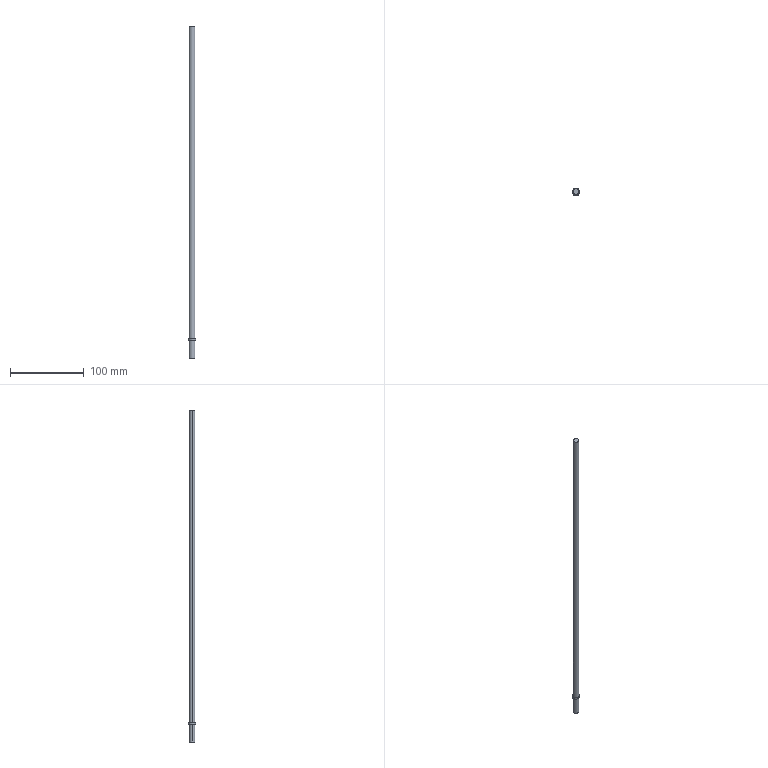Part | SolidWorks | features ICE 8, Extrusion 1 | 1 solid | 22 faces | box 10 x 10 x 449.1 mm | volume 22555 mm3 | cylinder 12 | plane 10 | commonest cylinder face diameters 3 x6 8 x4 10 x2
STEP:
#1=CARTESIAN_POINT('',(0.,2.2,447.1));
#2=VERTEX_POINT('',#1);
#3=CARTESIAN_POINT('',(1.5,2.2,445.6));
#4=VERTEX_POINT('',#3);
#5=CARTESIAN_POINT('',(0.,2.2,445.6));
#6=DIRECTION('',(0.,1.,0.));
#7=DIRECTION('',(0.,0.,1.));
#8=AXIS2_PLACEMENT_3D('',#5,#6,#7);
#9=CIRCLE('',#8,1.5);
#10=EDGE_CURVE('',#2,#4,#9,.T.);
#11=ORIENTED_EDGE('',*,*,#10,.F.);
#12=CARTESIAN_POINT('',(0.,4.,447.1));
#13=VERTEX_POINT('',#12);
#14=CARTESIAN_POINT('',(0.,2.2,447.1));
#15=DIRECTION('',(0.,1.,0.));
#16=VECTOR('',#15,1000.);
#17=LINE('',#14,#16);
#18=EDGE_CURVE('',#2,#13,#17,.T.);
#19=ORIENTED_EDGE('',*,*,#18,.T.);
#20=CARTESIAN_POINT('',(1.5,3.708,445.6));
#21=VERTEX_POINT('',#20);
#22=CARTESIAN_POINT('',(1.5,3.708,445.6));
#23=CARTESIAN_POINT('',(1.5,3.708,445.7));
#24=CARTESIAN_POINT('',(1.49,3.712,445.798));
#25=CARTESIAN_POINT('',(1.451,3.727,445.991));
#26=CARTESIAN_POINT('',(1.422,3.739,446.087));
#27=CARTESIAN_POINT('',(1.309,3.781,446.359));
#28=CARTESIAN_POINT('',(1.197,3.819,446.524));
#29=CARTESIAN_POINT('',(0.9232,3.895,446.798));
#30=CARTESIAN_POINT('',(0.7573,3.932,446.909));
#31=CARTESIAN_POINT('',(0.4867,3.971,447.022));
#32=CARTESIAN_POINT('',(0.3912,3.982,447.051));
#33=CARTESIAN_POINT('',(0.197,3.996,447.09));
#34=CARTESIAN_POINT('',(0.09895,4.,447.1));
#35=CARTESIAN_POINT('',(0.,4.,447.1));
#36=B_SPLINE_CURVE_WITH_KNOTS('',3,(#22,#23,#24,#25,#26,#27,#28,#29,#30,#31,#32,#33,#34,#35),.UNSPECIFIED.,.F.,.F.,(4,2,2,2,2,2,4),(0.,0.0002959,0.0005918,0.001184,0.001775,0.002071,0.002367),.UNSPECIFIED.);
#37=EDGE_CURVE('',#21,#13,#36,.T.);
#38=ORIENTED_EDGE('',*,*,#37,.F.);
#39=CARTESIAN_POINT('',(1.5,2.2,445.6));
#40=DIRECTION('',(0.,1.,0.));
#41=VECTOR('',#40,1000.);
#42=LINE('',#39,#41);
#43=EDGE_CURVE('',#4,#21,#42,.T.);
#44=ORIENTED_EDGE('',*,*,#43,.F.);
#45=EDGE_LOOP('',(#11,#19,#38,#44));
#46=FACE_OUTER_BOUND('',#45,.T.);
#47=CARTESIAN_POINT('',(0.,2.2,445.6));
#48=DIRECTION('',(0.,1.,0.));
#49=DIRECTION('',(0.,0.,1.));
#50=AXIS2_PLACEMENT_3D('',#47,#48,#49);
#51=CYLINDRICAL_SURFACE('',#50,1.5);
#52=ADVANCED_FACE('',(#46),#51,.F.);
#53=CARTESIAN_POINT('',(1.5,3.708,440.6));
#54=VERTEX_POINT('',#53);
#55=CARTESIAN_POINT('',(1.5,3.708,68.));
#56=DIRECTION('',(0.,0.,1.));
#57=VECTOR('',#56,1000.);
#58=LINE('',#55,#57);
#59=EDGE_CURVE('',#54,#21,#58,.T.);
#60=ORIENTED_EDGE('',*,*,#59,.T.);
#61=ORIENTED_EDGE('',*,*,#37,.T.);
#62=CARTESIAN_POINT('',(-1.5,3.708,445.6));
#63=VERTEX_POINT('',#62);
#64=CARTESIAN_POINT('',(0.,4.,447.1));
#65=CARTESIAN_POINT('',(-0.0988,4.,447.1));
#66=CARTESIAN_POINT('',(-0.1991,3.996,447.09));
#67=CARTESIAN_POINT('',(-0.3921,3.982,447.051));
#68=CARTESIAN_POINT('',(-0.486,3.971,447.023));
#69=CARTESIAN_POINT('',(-0.6687,3.945,446.946));
#70=CARTESIAN_POINT('',(-0.7547,3.929,446.9));
#71=CARTESIAN_POINT('',(-0.9162,3.895,446.792));
#72=CARTESIAN_POINT('',(-0.9924,3.876,446.729));
#73=CARTESIAN_POINT('',(-1.13,3.838,446.591));
#74=CARTESIAN_POINT('',(-1.191,3.819,446.517));
#75=CARTESIAN_POINT('',(-1.3,3.783,446.355));
#76=CARTESIAN_POINT('',(-1.347,3.767,446.268));
#77=CARTESIAN_POINT('',(-1.459,3.725,445.998));
#78=CARTESIAN_POINT('',(-1.5,3.708,445.8));
#79=CARTESIAN_POINT('',(-1.5,3.708,445.6));
#80=B_SPLINE_CURVE_WITH_KNOTS('',3,(#64,#65,#66,#67,#68,#69,#70,#71,#72,#73,#74,#75,#76,#77,#78,#79),.UNSPECIFIED.,.F.,.F.,(4,2,2,2,2,2,2,4),(0.002367,0.002663,0.002958,0.003254,0.003549,0.003845,0.00414,0.004731),.UNSPECIFIED.);
#81=EDGE_CURVE('',#13,#63,#80,.T.);
#82=ORIENTED_EDGE('',*,*,#81,.T.);
#83=CARTESIAN_POINT('',(-1.5,3.708,440.6));
#84=VERTEX_POINT('',#83);
#85=CARTESIAN_POINT('',(-1.5,3.708,68.));
#86=DIRECTION('',(0.,0.,-1.));
#87=VECTOR('',#86,1000.);
#88=LINE('',#85,#87);
#89=EDGE_CURVE('',#63,#84,#88,.T.);
#90=ORIENTED_EDGE('',*,*,#89,.T.);
#91=CARTESIAN_POINT('',(-1.5,3.708,440.6));
#92=CARTESIAN_POINT('',(-1.5,3.708,440.5));
#93=CARTESIAN_POINT('',(-1.49,3.712,440.402));
#94=CARTESIAN_POINT('',(-1.451,3.727,440.209));
#95=CARTESIAN_POINT('',(-1.422,3.739,440.113));
#96=CARTESIAN_POINT('',(-1.309,3.781,439.842));
#97=CARTESIAN_POINT('',(-1.198,3.819,439.677));
#98=CARTESIAN_POINT('',(-0.924,3.894,439.403));
#99=CARTESIAN_POINT('',(-0.7582,3.932,439.291));
#100=CARTESIAN_POINT('',(-0.488,3.971,439.178));
#101=CARTESIAN_POINT('',(-0.3926,3.982,439.149));
#102=CARTESIAN_POINT('',(-0.1986,3.996,439.11));
#103=CARTESIAN_POINT('',(-0.1006,4.,439.1));
#104=CARTESIAN_POINT('',(0.09712,4.,439.1));
#105=CARTESIAN_POINT('',(0.1975,3.996,439.11));
#106=CARTESIAN_POINT('',(0.3907,3.982,439.148));
#107=CARTESIAN_POINT('',(0.4847,3.972,439.177));
#108=CARTESIAN_POINT('',(0.759,3.932,439.291));
#109=CARTESIAN_POINT('',(0.9229,3.895,439.402));
#110=CARTESIAN_POINT('',(1.129,3.838,439.608));
#111=CARTESIAN_POINT('',(1.191,3.819,439.683));
#112=CARTESIAN_POINT('',(1.299,3.783,439.844));
#113=CARTESIAN_POINT('',(1.347,3.767,439.932));
#114=CARTESIAN_POINT('',(1.459,3.725,440.202));
#115=CARTESIAN_POINT('',(1.5,3.708,440.4));
#116=CARTESIAN_POINT('',(1.5,3.708,440.6));
#117=B_SPLINE_CURVE_WITH_KNOTS('',3,(#91,#92,#93,#94,#95,#96,#97,#98,#99,#100,#101,#102,#103,#104,#105,#106,#107,#108,#109,#110,#111,#112,#113,#114,#115,#116),.UNSPECIFIED.,.F.,.F.,(4,2,2,2,2,2,2,2,2,2,2,2,4),(0.,0.0002957,0.0005914,0.001183,0.001774,0.00207,0.002366,0.002661,0.002957,0.003548,0.003844,0.00414,0.004731),.UNSPECIFIED.);
#118=EDGE_CURVE('',#84,#54,#117,.T.);
#119=ORIENTED_EDGE('',*,*,#118,.T.);
#120=EDGE_LOOP('',(#60,#61,#82,#90,#119));
#121=FACE_BOUND('',#120,.T.);
#122=CARTESIAN_POINT('',(4.,0.,449.1));
#123=VERTEX_POINT('',#122);
#124=CARTESIAN_POINT('',(-4.,0.,449.1));
#125=VERTEX_POINT('',#124);
#126=CARTESIAN_POINT('',(0.,0.,449.1));
#127=DIRECTION('',(0.,0.,1.));
#128=DIRECTION('',(1.,0.,0.));
#129=AXIS2_PLACEMENT_3D('',#126,#127,#128);
#130=CIRCLE('',#129,4.);
#131=EDGE_CURVE('',#123,#125,#130,.T.);
#132=ORIENTED_EDGE('',*,*,#131,.F.);
#133=CARTESIAN_POINT('',(4.,0.,26.));
#134=VERTEX_POINT('',#133);
#135=CARTESIAN_POINT('',(4.,0.,68.));
#136=DIRECTION('',(0.,0.,-1.));
#137=VECTOR('',#136,1000.);
#138=LINE('',#135,#137);
#139=EDGE_CURVE('',#123,#134,#138,.T.);
#140=ORIENTED_EDGE('',*,*,#139,.T.);
#141=CARTESIAN_POINT('',(-4.,0.,26.));
#142=VERTEX_POINT('',#141);
#143=CARTESIAN_POINT('',(0.,0.,26.));
#144=DIRECTION('',(0.,0.,1.));
#145=DIRECTION('',(1.,0.,0.));
#146=AXIS2_PLACEMENT_3D('',#143,#144,#145);
#147=CIRCLE('',#146,4.);
#148=EDGE_CURVE('',#134,#142,#147,.T.);
#149=ORIENTED_EDGE('',*,*,#148,.T.);
#150=CARTESIAN_POINT('',(-4.,0.,68.));
#151=DIRECTION('',(0.,0.,-1.));
#152=VECTOR('',#151,1000.);
#153=LINE('',#150,#152);
#154=EDGE_CURVE('',#125,#142,#153,.T.);
#155=ORIENTED_EDGE('',*,*,#154,.F.);
#156=EDGE_LOOP('',(#132,#140,#149,#155));
#157=FACE_OUTER_BOUND('',#156,.T.);
#158=CARTESIAN_POINT('',(0.,0.,68.));
#159=DIRECTION('',(0.,0.,-1.));
#160=DIRECTION('',(-1.,0.,0.));
#161=AXIS2_PLACEMENT_3D('',#158,#159,#160);
#162=CYLINDRICAL_SURFACE('',#161,4.);
#163=ADVANCED_FACE('',(#121,#157),#162,.T.);
#164=CARTESIAN_POINT('',(0.,2.2,12.));
#165=VERTEX_POINT('',#164);
#166=CARTESIAN_POINT('',(1.5,2.2,10.5));
#167=VERTEX_POINT('',#166);
#168=CARTESIAN_POINT('',(0.,2.2,10.5));
#169=DIRECTION('',(0.,1.,0.));
#170=DIRECTION('',(0.,0.,1.));
#171=AXIS2_PLACEMENT_3D('',#168,#169,#170);
#172=CIRCLE('',#171,1.5);
#173=EDGE_CURVE('',#165,#167,#172,.T.);
#174=ORIENTED_EDGE('',*,*,#173,.F.);
#175=CARTESIAN_POINT('',(0.,4.,12.));
#176=VERTEX_POINT('',#175);
#177=CARTESIAN_POINT('',(0.,2.2,12.));
#178=DIRECTION('',(0.,1.,0.));
#179=VECTOR('',#178,1000.);
#180=LINE('',#177,#179);
#181=EDGE_CURVE('',#165,#176,#180,.T.);
#182=ORIENTED_EDGE('',*,*,#181,.T.);
#183=CARTESIAN_POINT('',(1.5,3.708,10.5));
#184=VERTEX_POINT('',#183);
#185=CARTESIAN_POINT('',(1.5,3.708,10.5));
#186=CARTESIAN_POINT('',(1.5,3.708,10.6));
#187=CARTESIAN_POINT('',(1.49,3.712,10.698));
#188=CARTESIAN_POINT('',(1.451,3.727,10.891));
#189=CARTESIAN_POINT('',(1.422,3.739,10.987));
#190=CARTESIAN_POINT('',(1.309,3.781,11.259));
#191=CARTESIAN_POINT('',(1.197,3.819,11.424));
#192=CARTESIAN_POINT('',(0.9232,3.895,11.698));
#193=CARTESIAN_POINT('',(0.7573,3.932,11.809));
#194=CARTESIAN_POINT('',(0.4867,3.971,11.922));
#195=CARTESIAN_POINT('',(0.3912,3.982,11.951));
#196=CARTESIAN_POINT('',(0.197,3.996,11.99));
#197=CARTESIAN_POINT('',(0.09895,4.,12.));
#198=CARTESIAN_POINT('',(0.,4.,12.));
#199=B_SPLINE_CURVE_WITH_KNOTS('',3,(#185,#186,#187,#188,#189,#190,#191,#192,#193,#194,#195,#196,#197,#198),.UNSPECIFIED.,.F.,.F.,(4,2,2,2,2,2,4),(0.,0.0002959,0.0005918,0.001184,0.001775,0.002071,0.002367),.UNSPECIFIED.);
#200=EDGE_CURVE('',#184,#176,#199,.T.);
#201=ORIENTED_EDGE('',*,*,#200,.F.);
#202=CARTESIAN_POINT('',(1.5,2.2,10.5));
#203=DIRECTION('',(0.,1.,0.));
#204=VECTOR('',#203,1000.);
#205=LINE('',#202,#204);
#206=EDGE_CURVE('',#167,#184,#205,.T.);
#207=ORIENTED_EDGE('',*,*,#206,.F.);
#208=EDGE_LOOP('',(#174,#182,#201,#207));
#209=FACE_OUTER_BOUND('',#208,.T.);
#210=CARTESIAN_POINT('',(0.,2.2,10.5));
#211=DIRECTION('',(0.,1.,0.));
#212=DIRECTION('',(0.,0.,1.));
#213=AXIS2_PLACEMENT_3D('',#210,#211,#212);
#214=CYLINDRICAL_SURFACE('',#213,1.5);
#215=ADVANCED_FACE('',(#209),#214,.F.);
#216=CARTESIAN_POINT('',(5.,0.,26.));
#217=VERTEX_POINT('',#216);
#218=CARTESIAN_POINT('',(-5.,0.,26.));
#219=VERTEX_POINT('',#218);
#220=CARTESIAN_POINT('',(0.,0.,26.));
#221=DIRECTION('',(0.,0.,1.));
#222=DIRECTION('',(1.,0.,0.));
#223=AXIS2_PLACEMENT_3D('',#220,#221,#222);
#224=CIRCLE('',#223,5.);
#225=EDGE_CURVE('',#217,#219,#224,.T.);
#226=ORIENTED_EDGE('',*,*,#225,.F.);
#227=CARTESIAN_POINT('',(5.,0.,24.));
#228=VERTEX_POINT('',#227);
#229=CARTESIAN_POINT('',(5.,0.,26.));
#230=DIRECTION('',(0.,0.,-1.));
#231=VECTOR('',#230,1000.);
#232=LINE('',#229,#231);
#233=EDGE_CURVE('',#217,#228,#232,.T.);
#234=ORIENTED_EDGE('',*,*,#233,.T.);
#235=CARTESIAN_POINT('',(-5.,0.,24.));
#236=VERTEX_POINT('',#235);
#237=CARTESIAN_POINT('',(0.,0.,24.));
#238=DIRECTION('',(0.,0.,1.));
#239=DIRECTION('',(1.,0.,0.));
#240=AXIS2_PLACEMENT_3D('',#237,#238,#239);
#241=CIRCLE('',#240,5.);
#242=EDGE_CURVE('',#228,#236,#241,.T.);
#243=ORIENTED_EDGE('',*,*,#242,.T.);
#244=CARTESIAN_POINT('',(-5.,0.,26.));
#245=DIRECTION('',(0.,0.,-1.));
#246=VECTOR('',#245,1000.);
#247=LINE('',#244,#246);
#248=EDGE_CURVE('',#219,#236,#247,.T.);
#249=ORIENTED_EDGE('',*,*,#248,.F.);
#250=EDGE_LOOP('',(#226,#234,#243,#249));
#251=FACE_OUTER_BOUND('',#250,.T.);
#252=CARTESIAN_POINT('',(0.,0.,26.));
#253=DIRECTION('',(0.,0.,-1.));
#254=DIRECTION('',(-1.,0.,0.));
#255=AXIS2_PLACEMENT_3D('',#252,#253,#254);
#256=CYLINDRICAL_SURFACE('',#255,5.);
#257=ADVANCED_FACE('',(#251),#256,.T.);
#258=CARTESIAN_POINT('',(1.5,3.708,5.5));
#259=VERTEX_POINT('',#258);
#260=CARTESIAN_POINT('',(1.5,3.708,14.));
#261=DIRECTION('',(0.,0.,1.));
#262=VECTOR('',#261,1000.);
#263=LINE('',#260,#262);
#264=EDGE_CURVE('',#259,#184,#263,.T.);
#265=ORIENTED_EDGE('',*,*,#264,.T.);
#266=ORIENTED_EDGE('',*,*,#200,.T.);
#267=CARTESIAN_POINT('',(-1.5,3.708,10.5));
#268=VERTEX_POINT('',#267);
#269=CARTESIAN_POINT('',(0.,4.,12.));
#270=CARTESIAN_POINT('',(-0.0988,4.,12.));
#271=CARTESIAN_POINT('',(-0.1991,3.996,11.99));
#272=CARTESIAN_POINT('',(-0.3921,3.982,11.951));
#273=CARTESIAN_POINT('',(-0.486,3.971,11.923));
#274=CARTESIAN_POINT('',(-0.6687,3.945,11.846));
#275=CARTESIAN_POINT('',(-0.7547,3.929,11.8));
#276=CARTESIAN_POINT('',(-0.9162,3.895,11.692));
#277=CARTESIAN_POINT('',(-0.9924,3.876,11.629));
#278=CARTESIAN_POINT('',(-1.13,3.838,11.491));
#279=CARTESIAN_POINT('',(-1.191,3.819,11.417));
#280=CARTESIAN_POINT('',(-1.3,3.783,11.255));
#281=CARTESIAN_POINT('',(-1.347,3.767,11.168));
#282=CARTESIAN_POINT('',(-1.459,3.725,10.898));
#283=CARTESIAN_POINT('',(-1.5,3.708,10.7));
#284=CARTESIAN_POINT('',(-1.5,3.708,10.5));
#285=B_SPLINE_CURVE_WITH_KNOTS('',3,(#269,#270,#271,#272,#273,#274,#275,#276,#277,#278,#279,#280,#281,#282,#283,#284),.UNSPECIFIED.,.F.,.F.,(4,2,2,2,2,2,2,4),(0.002367,0.002663,0.002958,0.003254,0.003549,0.003845,0.00414,0.004731),.UNSPECIFIED.);
#286=EDGE_CURVE('',#176,#268,#285,.T.);
#287=ORIENTED_EDGE('',*,*,#286,.T.);
#288=CARTESIAN_POINT('',(-1.5,3.708,5.5));
#289=VERTEX_POINT('',#288);
#290=CARTESIAN_POINT('',(-1.5,3.708,14.));
#291=DIRECTION('',(0.,0.,-1.));
#292=VECTOR('',#291,1000.);
#293=LINE('',#290,#292);
#294=EDGE_CURVE('',#268,#289,#293,.T.);
#295=ORIENTED_EDGE('',*,*,#294,.T.);
#296=CARTESIAN_POINT('',(-1.5,3.708,5.5));
#297=CARTESIAN_POINT('',(-1.5,3.708,5.4));
#298=CARTESIAN_POINT('',(-1.49,3.712,5.302));
#299=CARTESIAN_POINT('',(-1.451,3.727,5.109));
#300=CARTESIAN_POINT('',(-1.422,3.739,5.013));
#301=CARTESIAN_POINT('',(-1.309,3.781,4.742));
#302=CARTESIAN_POINT('',(-1.198,3.819,4.577));
#303=CARTESIAN_POINT('',(-0.924,3.894,4.303));
#304=CARTESIAN_POINT('',(-0.7582,3.932,4.191));
#305=CARTESIAN_POINT('',(-0.488,3.971,4.078));
#306=CARTESIAN_POINT('',(-0.3926,3.982,4.049));
#307=CARTESIAN_POINT('',(-0.1986,3.996,4.01));
#308=CARTESIAN_POINT('',(-0.1006,4.,4.));
#309=CARTESIAN_POINT('',(0.09712,4.,4.));
#310=CARTESIAN_POINT('',(0.1975,3.996,4.01));
#311=CARTESIAN_POINT('',(0.3907,3.982,4.048));
#312=CARTESIAN_POINT('',(0.4847,3.972,4.077));
#313=CARTESIAN_POINT('',(0.759,3.932,4.191));
#314=CARTESIAN_POINT('',(0.9229,3.895,4.302));
#315=CARTESIAN_POINT('',(1.129,3.838,4.508));
#316=CARTESIAN_POINT('',(1.191,3.819,4.583));
#317=CARTESIAN_POINT('',(1.299,3.783,4.744));
#318=CARTESIAN_POINT('',(1.347,3.767,4.832));
#319=CARTESIAN_POINT('',(1.459,3.725,5.102));
#320=CARTESIAN_POINT('',(1.5,3.708,5.3));
#321=CARTESIAN_POINT('',(1.5,3.708,5.5));
#322=B_SPLINE_CURVE_WITH_KNOTS('',3,(#296,#297,#298,#299,#300,#301,#302,#303,#304,#305,#306,#307,#308,#309,#310,#311,#312,#313,#314,#315,#316,#317,#318,#319,#320,#321),.UNSPECIFIED.,.F.,.F.,(4,2,2,2,2,2,2,2,2,2,2,2,4),(0.,0.0002957,0.0005914,0.001183,0.001774,0.00207,0.002366,0.002661,0.002957,0.003548,0.003844,0.00414,0.004731),.UNSPECIFIED.);
#323=EDGE_CURVE('',#289,#259,#322,.T.);
#324=ORIENTED_EDGE('',*,*,#323,.T.);
#325=EDGE_LOOP('',(#265,#266,#287,#295,#324));
#326=FACE_BOUND('',#325,.T.);
#327=CARTESIAN_POINT('',(4.,0.,24.));
#328=VERTEX_POINT('',#327);
#329=CARTESIAN_POINT('',(-4.,0.,24.));
#330=VERTEX_POINT('',#329);
#331=CARTESIAN_POINT('',(0.,0.,24.));
#332=DIRECTION('',(0.,0.,1.));
#333=DIRECTION('',(1.,0.,0.));
#334=AXIS2_PLACEMENT_3D('',#331,#332,#333);
#335=CIRCLE('',#334,4.);
#336=EDGE_CURVE('',#328,#330,#335,.T.);
#337=ORIENTED_EDGE('',*,*,#336,.F.);
#338=CARTESIAN_POINT('',(4.,0.,0.));
#339=VERTEX_POINT('',#338);
#340=CARTESIAN_POINT('',(4.,0.,14.));
#341=DIRECTION('',(0.,0.,-1.));
#342=VECTOR('',#341,1000.);
#343=LINE('',#340,#342);
#344=EDGE_CURVE('',#328,#339,#343,.T.);
#345=ORIENTED_EDGE('',*,*,#344,.T.);
#346=CARTESIAN_POINT('',(-4.,0.,0.));
#347=VERTEX_POINT('',#346);
#348=CARTESIAN_POINT('',(0.,0.,0.));
#349=DIRECTION('',(0.,0.,1.));
#350=DIRECTION('',(1.,0.,0.));
#351=AXIS2_PLACEMENT_3D('',#348,#349,#350);
#352=CIRCLE('',#351,4.);
#353=EDGE_CURVE('',#339,#347,#352,.T.);
#354=ORIENTED_EDGE('',*,*,#353,.T.);
#355=CARTESIAN_POINT('',(-4.,0.,14.));
#356=DIRECTION('',(0.,0.,-1.));
#357=VECTOR('',#356,1000.);
#358=LINE('',#355,#357);
#359=EDGE_CURVE('',#330,#347,#358,.T.);
#360=ORIENTED_EDGE('',*,*,#359,.F.);
#361=EDGE_LOOP('',(#337,#345,#354,#360));
#362=FACE_OUTER_BOUND('',#361,.T.);
#363=CARTESIAN_POINT('',(0.,0.,14.));
#364=DIRECTION('',(0.,0.,-1.));
#365=DIRECTION('',(-1.,0.,0.));
#366=AXIS2_PLACEMENT_3D('',#363,#364,#365);
#367=CYLINDRICAL_SURFACE('',#366,4.);
#368=ADVANCED_FACE('',(#326,#362),#367,.T.);
#369=ORIENTED_EDGE('',*,*,#344,.F.);
#370=CARTESIAN_POINT('',(0.,0.,24.));
#371=DIRECTION('',(0.,0.,1.));
#372=DIRECTION('',(1.,0.,0.));
#373=AXIS2_PLACEMENT_3D('',#370,#371,#372);
#374=CIRCLE('',#373,4.);
#375=EDGE_CURVE('',#330,#328,#374,.T.);
#376=ORIENTED_EDGE('',*,*,#375,.F.);
#377=ORIENTED_EDGE('',*,*,#359,.T.);
#378=CARTESIAN_POINT('',(0.,0.,0.));
#379=DIRECTION('',(0.,0.,1.));
#380=DIRECTION('',(1.,0.,0.));
#381=AXIS2_PLACEMENT_3D('',#378,#379,#380);
#382=CIRCLE('',#381,4.);
#383=EDGE_CURVE('',#347,#339,#382,.T.);
#384=ORIENTED_EDGE('',*,*,#383,.T.);
#385=EDGE_LOOP('',(#369,#376,#377,#384));
#386=FACE_OUTER_BOUND('',#385,.T.);
#387=CARTESIAN_POINT('',(0.,0.,14.));
#388=DIRECTION('',(0.,0.,-1.));
#389=DIRECTION('',(-1.,0.,0.));
#390=AXIS2_PLACEMENT_3D('',#387,#388,#389);
#391=CYLINDRICAL_SURFACE('',#390,4.);
#392=ADVANCED_FACE('',(#386),#391,.T.);
#393=ORIENTED_EDGE('',*,*,#383,.F.);
#394=ORIENTED_EDGE('',*,*,#353,.F.);
#395=EDGE_LOOP('',(#393,#394));
#396=FACE_OUTER_BOUND('',#395,.T.);
#397=CARTESIAN_POINT('',(0.,0.,0.));
#398=DIRECTION('',(0.,0.,1.));
#399=DIRECTION('',(1.,0.,0.));
#400=AXIS2_PLACEMENT_3D('',#397,#398,#399);
#401=PLANE('',#400);
#402=ADVANCED_FACE('',(#396),#401,.F.);
#403=ORIENTED_EDGE('',*,*,#233,.F.);
#404=CARTESIAN_POINT('',(0.,0.,26.));
#405=DIRECTION('',(0.,0.,1.));
#406=DIRECTION('',(1.,0.,0.));
#407=AXIS2_PLACEMENT_3D('',#404,#405,#406);
#408=CIRCLE('',#407,5.);
#409=EDGE_CURVE('',#219,#217,#408,.T.);
#410=ORIENTED_EDGE('',*,*,#409,.F.);
#411=ORIENTED_EDGE('',*,*,#248,.T.);
#412=CARTESIAN_POINT('',(0.,0.,24.));
#413=DIRECTION('',(0.,0.,1.));
#414=DIRECTION('',(1.,0.,0.));
#415=AXIS2_PLACEMENT_3D('',#412,#413,#414);
#416=CIRCLE('',#415,5.);
#417=EDGE_CURVE('',#236,#228,#416,.T.);
#418=ORIENTED_EDGE('',*,*,#417,.T.);
#419=EDGE_LOOP('',(#403,#410,#411,#418));
#420=FACE_OUTER_BOUND('',#419,.T.);
#421=CARTESIAN_POINT('',(0.,0.,26.));
#422=DIRECTION('',(0.,0.,-1.));
#423=DIRECTION('',(-1.,0.,0.));
#424=AXIS2_PLACEMENT_3D('',#421,#422,#423);
#425=CYLINDRICAL_SURFACE('',#424,5.);
#426=ADVANCED_FACE('',(#420),#425,.T.);
#427=CARTESIAN_POINT('',(0.,0.,26.));
#428=DIRECTION('',(0.,0.,1.));
#429=DIRECTION('',(1.,0.,0.));
#430=AXIS2_PLACEMENT_3D('',#427,#428,#429);
#431=CIRCLE('',#430,4.);
#432=EDGE_CURVE('',#142,#134,#431,.T.);
#433=ORIENTED_EDGE('',*,*,#432,.F.);
#434=ORIENTED_EDGE('',*,*,#148,.F.);
#435=EDGE_LOOP('',(#433,#434));
#436=FACE_BOUND('',#435,.T.);
#437=ORIENTED_EDGE('',*,*,#409,.T.);
#438=ORIENTED_EDGE('',*,*,#225,.T.);
#439=EDGE_LOOP('',(#437,#438));
#440=FACE_OUTER_BOUND('',#439,.T.);
#441=CARTESIAN_POINT('',(0.,0.,26.));
#442=DIRECTION('',(0.,0.,1.));
#443=DIRECTION('',(1.,0.,0.));
#444=AXIS2_PLACEMENT_3D('',#441,#442,#443);
#445=PLANE('',#444);
#446=ADVANCED_FACE('',(#436,#440),#445,.T.);
#447=ORIENTED_EDGE('',*,*,#375,.T.);
#448=ORIENTED_EDGE('',*,*,#336,.T.);
#449=EDGE_LOOP('',(#447,#448));
#450=FACE_BOUND('',#449,.T.);
#451=ORIENTED_EDGE('',*,*,#417,.F.);
#452=ORIENTED_EDGE('',*,*,#242,.F.);
#453=EDGE_LOOP('',(#451,#452));
#454=FACE_OUTER_BOUND('',#453,.T.);
#455=CARTESIAN_POINT('',(0.,0.,24.));
#456=DIRECTION('',(0.,0.,1.));
#457=DIRECTION('',(1.,0.,0.));
#458=AXIS2_PLACEMENT_3D('',#455,#456,#457);
#459=PLANE('',#458);
#460=ADVANCED_FACE('',(#450,#454),#459,.F.);
#461=CARTESIAN_POINT('',(-1.5,2.2,5.5));
#462=VERTEX_POINT('',#461);
#463=CARTESIAN_POINT('',(-1.5,2.2,5.5));
#464=DIRECTION('',(0.,1.,0.));
#465=VECTOR('',#464,1000.);
#466=LINE('',#463,#465);
#467=EDGE_CURVE('',#462,#289,#466,.T.);
#468=ORIENTED_EDGE('',*,*,#467,.F.);
#469=CARTESIAN_POINT('',(1.5,2.2,5.5));
#470=VERTEX_POINT('',#469);
#471=CARTESIAN_POINT('',(0.,2.2,5.5));
#472=DIRECTION('',(0.,1.,0.));
#473=DIRECTION('',(0.,0.,1.));
#474=AXIS2_PLACEMENT_3D('',#471,#472,#473);
#475=CIRCLE('',#474,1.5);
#476=EDGE_CURVE('',#470,#462,#475,.T.);
#477=ORIENTED_EDGE('',*,*,#476,.F.);
#478=CARTESIAN_POINT('',(1.5,2.2,5.5));
#479=DIRECTION('',(0.,1.,0.));
#480=VECTOR('',#479,1000.);
#481=LINE('',#478,#480);
#482=EDGE_CURVE('',#470,#259,#481,.T.);
#483=ORIENTED_EDGE('',*,*,#482,.T.);
#484=ORIENTED_EDGE('',*,*,#323,.F.);
#485=EDGE_LOOP('',(#468,#477,#483,#484));
#486=FACE_OUTER_BOUND('',#485,.T.);
#487=CARTESIAN_POINT('',(0.,2.2,5.5));
#488=DIRECTION('',(0.,1.,0.));
#489=DIRECTION('',(0.,0.,1.));
#490=AXIS2_PLACEMENT_3D('',#487,#488,#489);
#491=CYLINDRICAL_SURFACE('',#490,1.5);
#492=ADVANCED_FACE('',(#486),#491,.F.);
#493=ORIENTED_EDGE('',*,*,#482,.F.);
#494=CARTESIAN_POINT('',(1.5,2.2,5.5));
#495=DIRECTION('',(0.,0.,-1.));
#496=VECTOR('',#495,1000.);
#497=LINE('',#494,#496);
#498=EDGE_CURVE('',#167,#470,#497,.T.);
#499=ORIENTED_EDGE('',*,*,#498,.F.);
#500=ORIENTED_EDGE('',*,*,#206,.T.);
#501=ORIENTED_EDGE('',*,*,#264,.F.);
#502=EDGE_LOOP('',(#493,#499,#500,#501));
#503=FACE_OUTER_BOUND('',#502,.T.);
#504=CARTESIAN_POINT('',(1.5,2.2,5.5));
#505=DIRECTION('',(1.,0.,0.));
#506=DIRECTION('',(0.,0.,-1.));
#507=AXIS2_PLACEMENT_3D('',#504,#505,#506);
#508=PLANE('',#507);
#509=ADVANCED_FACE('',(#503),#508,.F.);
#510=ORIENTED_EDGE('',*,*,#181,.F.);
#511=CARTESIAN_POINT('',(-1.5,2.2,10.5));
#512=VERTEX_POINT('',#511);
#513=CARTESIAN_POINT('',(0.,2.2,10.5));
#514=DIRECTION('',(0.,1.,0.));
#515=DIRECTION('',(0.,0.,1.));
#516=AXIS2_PLACEMENT_3D('',#513,#514,#515);
#517=CIRCLE('',#516,1.5);
#518=EDGE_CURVE('',#512,#165,#517,.T.);
#519=ORIENTED_EDGE('',*,*,#518,.F.);
#520=CARTESIAN_POINT('',(-1.5,2.2,10.5));
#521=DIRECTION('',(0.,1.,0.));
#522=VECTOR('',#521,1000.);
#523=LINE('',#520,#522);
#524=EDGE_CURVE('',#512,#268,#523,.T.);
#525=ORIENTED_EDGE('',*,*,#524,.T.);
#526=ORIENTED_EDGE('',*,*,#286,.F.);
#527=EDGE_LOOP('',(#510,#519,#525,#526));
#528=FACE_OUTER_BOUND('',#527,.T.);
#529=CARTESIAN_POINT('',(0.,2.2,10.5));
#530=DIRECTION('',(0.,1.,0.));
#531=DIRECTION('',(0.,0.,1.));
#532=AXIS2_PLACEMENT_3D('',#529,#530,#531);
#533=CYLINDRICAL_SURFACE('',#532,1.5);
#534=ADVANCED_FACE('',(#528),#533,.F.);
#535=ORIENTED_EDGE('',*,*,#524,.F.);
#536=CARTESIAN_POINT('',(-1.5,2.2,5.5));
#537=DIRECTION('',(0.,0.,1.));
#538=VECTOR('',#537,1000.);
#539=LINE('',#536,#538);
#540=EDGE_CURVE('',#462,#512,#539,.T.);
#541=ORIENTED_EDGE('',*,*,#540,.F.);
#542=ORIENTED_EDGE('',*,*,#467,.T.);
#543=ORIENTED_EDGE('',*,*,#294,.F.);
#544=EDGE_LOOP('',(#535,#541,#542,#543));
#545=FACE_OUTER_BOUND('',#544,.T.);
#546=CARTESIAN_POINT('',(-1.5,2.2,5.5));
#547=DIRECTION('',(-1.,0.,0.));
#548=DIRECTION('',(0.,0.,1.));
#549=AXIS2_PLACEMENT_3D('',#546,#547,#548);
#550=PLANE('',#549);
#551=ADVANCED_FACE('',(#545),#550,.F.);
#552=ORIENTED_EDGE('',*,*,#476,.T.);
#553=ORIENTED_EDGE('',*,*,#540,.T.);
#554=ORIENTED_EDGE('',*,*,#518,.T.);
#555=ORIENTED_EDGE('',*,*,#173,.T.);
#556=ORIENTED_EDGE('',*,*,#498,.T.);
#557=EDGE_LOOP('',(#552,#553,#554,#555,#556));
#558=FACE_OUTER_BOUND('',#557,.T.);
#559=CARTESIAN_POINT('',(0.,2.2,5.5));
#560=DIRECTION('',(0.,1.,0.));
#561=DIRECTION('',(0.,0.,1.));
#562=AXIS2_PLACEMENT_3D('',#559,#560,#561);
#563=PLANE('',#562);
#564=ADVANCED_FACE('',(#558),#563,.T.);
#565=ORIENTED_EDGE('',*,*,#139,.F.);
#566=CARTESIAN_POINT('',(0.,0.,449.1));
#567=DIRECTION('',(0.,0.,1.));
#568=DIRECTION('',(1.,0.,0.));
#569=AXIS2_PLACEMENT_3D('',#566,#567,#568);
#570=CIRCLE('',#569,4.);
#571=EDGE_CURVE('',#125,#123,#570,.T.);
#572=ORIENTED_EDGE('',*,*,#571,.F.);
#573=ORIENTED_EDGE('',*,*,#154,.T.);
#574=ORIENTED_EDGE('',*,*,#432,.T.);
#575=EDGE_LOOP('',(#565,#572,#573,#574));
#576=FACE_OUTER_BOUND('',#575,.T.);
#577=CARTESIAN_POINT('',(0.,0.,68.));
#578=DIRECTION('',(0.,0.,-1.));
#579=DIRECTION('',(-1.,0.,0.));
#580=AXIS2_PLACEMENT_3D('',#577,#578,#579);
#581=CYLINDRICAL_SURFACE('',#580,4.);
#582=ADVANCED_FACE('',(#576),#581,.T.);
#583=ORIENTED_EDGE('',*,*,#571,.T.);
#584=ORIENTED_EDGE('',*,*,#131,.T.);
#585=EDGE_LOOP('',(#583,#584));
#586=FACE_OUTER_BOUND('',#585,.T.);
#587=CARTESIAN_POINT('',(0.,0.,449.1));
#588=DIRECTION('',(0.,0.,1.));
#589=DIRECTION('',(1.,0.,0.));
#590=AXIS2_PLACEMENT_3D('',#587,#588,#589);
#591=PLANE('',#590);
#592=ADVANCED_FACE('',(#586),#591,.T.);
#593=CARTESIAN_POINT('',(-1.5,2.2,440.6));
#594=VERTEX_POINT('',#593);
#595=CARTESIAN_POINT('',(-1.5,2.2,440.6));
#596=DIRECTION('',(0.,1.,0.));
#597=VECTOR('',#596,1000.);
#598=LINE('',#595,#597);
#599=EDGE_CURVE('',#594,#84,#598,.T.);
#600=ORIENTED_EDGE('',*,*,#599,.F.);
#601=CARTESIAN_POINT('',(1.5,2.2,440.6));
#602=VERTEX_POINT('',#601);
#603=CARTESIAN_POINT('',(0.,2.2,440.6));
#604=DIRECTION('',(0.,1.,0.));
#605=DIRECTION('',(0.,0.,1.));
#606=AXIS2_PLACEMENT_3D('',#603,#604,#605);
#607=CIRCLE('',#606,1.5);
#608=EDGE_CURVE('',#602,#594,#607,.T.);
#609=ORIENTED_EDGE('',*,*,#608,.F.);
#610=CARTESIAN_POINT('',(1.5,2.2,440.6));
#611=DIRECTION('',(0.,1.,0.));
#612=VECTOR('',#611,1000.);
#613=LINE('',#610,#612);
#614=EDGE_CURVE('',#602,#54,#613,.T.);
#615=ORIENTED_EDGE('',*,*,#614,.T.);
#616=ORIENTED_EDGE('',*,*,#118,.F.);
#617=EDGE_LOOP('',(#600,#609,#615,#616));
#618=FACE_OUTER_BOUND('',#617,.T.);
#619=CARTESIAN_POINT('',(0.,2.2,440.6));
#620=DIRECTION('',(0.,1.,0.));
#621=DIRECTION('',(0.,0.,1.));
#622=AXIS2_PLACEMENT_3D('',#619,#620,#621);
#623=CYLINDRICAL_SURFACE('',#622,1.5);
#624=ADVANCED_FACE('',(#618),#623,.F.);
#625=ORIENTED_EDGE('',*,*,#614,.F.);
#626=CARTESIAN_POINT('',(1.5,2.2,440.6));
#627=DIRECTION('',(0.,0.,-1.));
#628=VECTOR('',#627,1000.);
#629=LINE('',#626,#628);
#630=EDGE_CURVE('',#4,#602,#629,.T.);
#631=ORIENTED_EDGE('',*,*,#630,.F.);
#632=ORIENTED_EDGE('',*,*,#43,.T.);
#633=ORIENTED_EDGE('',*,*,#59,.F.);
#634=EDGE_LOOP('',(#625,#631,#632,#633));
#635=FACE_OUTER_BOUND('',#634,.T.);
#636=CARTESIAN_POINT('',(1.5,2.2,440.6));
#637=DIRECTION('',(1.,0.,0.));
#638=DIRECTION('',(0.,0.,-1.));
#639=AXIS2_PLACEMENT_3D('',#636,#637,#638);
#640=PLANE('',#639);
#641=ADVANCED_FACE('',(#635),#640,.F.);
#642=ORIENTED_EDGE('',*,*,#18,.F.);
#643=CARTESIAN_POINT('',(-1.5,2.2,445.6));
#644=VERTEX_POINT('',#643);
#645=CARTESIAN_POINT('',(0.,2.2,445.6));
#646=DIRECTION('',(0.,1.,0.));
#647=DIRECTION('',(0.,0.,1.));
#648=AXIS2_PLACEMENT_3D('',#645,#646,#647);
#649=CIRCLE('',#648,1.5);
#650=EDGE_CURVE('',#644,#2,#649,.T.);
#651=ORIENTED_EDGE('',*,*,#650,.F.);
#652=CARTESIAN_POINT('',(-1.5,2.2,445.6));
#653=DIRECTION('',(0.,1.,0.));
#654=VECTOR('',#653,1000.);
#655=LINE('',#652,#654);
#656=EDGE_CURVE('',#644,#63,#655,.T.);
#657=ORIENTED_EDGE('',*,*,#656,.T.);
#658=ORIENTED_EDGE('',*,*,#81,.F.);
#659=EDGE_LOOP('',(#642,#651,#657,#658));
#660=FACE_OUTER_BOUND('',#659,.T.);
#661=CARTESIAN_POINT('',(0.,2.2,445.6));
#662=DIRECTION('',(0.,1.,0.));
#663=DIRECTION('',(0.,0.,1.));
#664=AXIS2_PLACEMENT_3D('',#661,#662,#663);
#665=CYLINDRICAL_SURFACE('',#664,1.5);
#666=ADVANCED_FACE('',(#660),#665,.F.);
#667=ORIENTED_EDGE('',*,*,#656,.F.);
#668=CARTESIAN_POINT('',(-1.5,2.2,440.6));
#669=DIRECTION('',(0.,0.,1.));
#670=VECTOR('',#669,1000.);
#671=LINE('',#668,#670);
#672=EDGE_CURVE('',#594,#644,#671,.T.);
#673=ORIENTED_EDGE('',*,*,#672,.F.);
#674=ORIENTED_EDGE('',*,*,#599,.T.);
#675=ORIENTED_EDGE('',*,*,#89,.F.);
#676=EDGE_LOOP('',(#667,#673,#674,#675));
#677=FACE_OUTER_BOUND('',#676,.T.);
#678=CARTESIAN_POINT('',(-1.5,2.2,440.6));
#679=DIRECTION('',(-1.,0.,0.));
#680=DIRECTION('',(0.,0.,1.));
#681=AXIS2_PLACEMENT_3D('',#678,#679,#680);
#682=PLANE('',#681);
#683=ADVANCED_FACE('',(#677),#682,.F.);
#684=ORIENTED_EDGE('',*,*,#608,.T.);
#685=ORIENTED_EDGE('',*,*,#672,.T.);
#686=ORIENTED_EDGE('',*,*,#650,.T.);
#687=ORIENTED_EDGE('',*,*,#10,.T.);
#688=ORIENTED_EDGE('',*,*,#630,.T.);
#689=EDGE_LOOP('',(#684,#685,#686,#687,#688));
#690=FACE_OUTER_BOUND('',#689,.T.);
#691=CARTESIAN_POINT('',(0.,2.2,440.6));
#692=DIRECTION('',(0.,1.,0.));
#693=DIRECTION('',(0.,0.,1.));
#694=AXIS2_PLACEMENT_3D('',#691,#692,#693);
#695=PLANE('',#694);
#696=ADVANCED_FACE('',(#690),#695,.T.);
#697=CLOSED_SHELL('',(#52,#163,#215,#257,#368,#392,#402,#426,#446,#460,#492,#509,#534,#551,#564,#582,#592,#624,#641,#666,#683,#696));
#698=MANIFOLD_SOLID_BREP('',#697);
#699=CARTESIAN_POINT('',(0.,0.,0.));
#700=DIRECTION('',(0.,0.,1.));
#701=DIRECTION('',(1.,0.,0.));
#702=AXIS2_PLACEMENT_3D('',#699,#700,#701);
#703=(LENGTH_UNIT()NAMED_UNIT(*)SI_UNIT(.MILLI.,.METRE.));
#704=UNCERTAINTY_MEASURE_WITH_UNIT(LENGTH_MEASURE(0.00001),#703,'','');
#705=(NAMED_UNIT(*)PLANE_ANGLE_UNIT()SI_UNIT($,.RADIAN.));
#706=(NAMED_UNIT(*)SI_UNIT($,.STERADIAN.)SOLID_ANGLE_UNIT());
#707=(GEOMETRIC_REPRESENTATION_CONTEXT(3)GLOBAL_UNCERTAINTY_ASSIGNED_CONTEXT((#704))GLOBAL_UNIT_ASSIGNED_CONTEXT((#703,#705,#706))REPRESENTATION_CONTEXT('',''));
#708=ADVANCED_BREP_SHAPE_REPRESENTATION('',(#698,#702),#707);